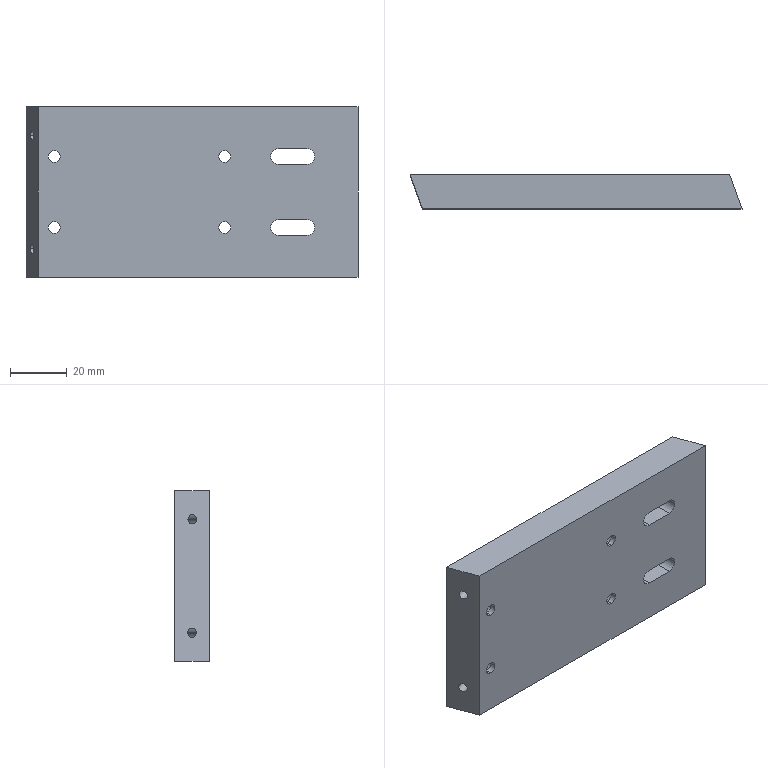Part | STEP file | vibratory feeder upper plate | 1 solid | 64 faces | box 116.996 x 12 x 60 mm | volume 77221 mm3 | cylinder 36 | plane 20 | cone 8 | commonest cylinder face diameters 3.3 x8 4.2 x8 5 x8 5.5 x6 9 x6